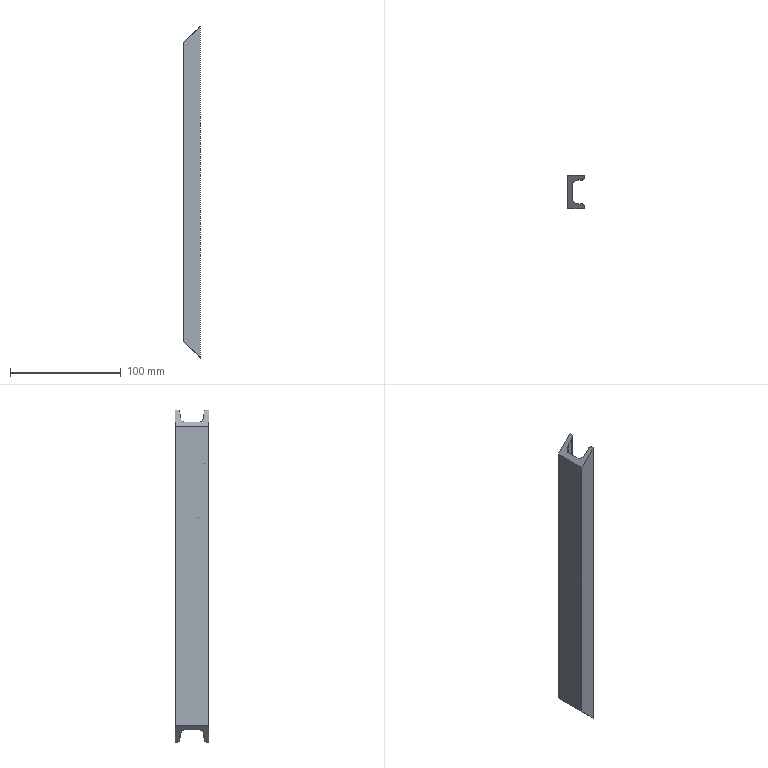Part | STEP file | DIN 1026-1 U 30x15 1785506933780 | 1 solid | 14 faces | box 15 x 30 x 300 mm | volume 62027 mm3 | plane 10 | cylinder 4 | commonest cylinder face diameters 4 x2 9 x2
STEP:
#1=CARTESIAN_POINT('',(13.159,-10.953,283.159));
#2=VERTEX_POINT('',#1);
#3=CARTESIAN_POINT('',(15.,-12.946,285.));
#4=VERTEX_POINT('',#3);
#5=CARTESIAN_POINT('',(13.,-12.946,283.));
#6=DIRECTION('',(0.7071,0.,-0.7071));
#7=DIRECTION('',(-0.7071,0.,-0.7071));
#8=AXIS2_PLACEMENT_3D('',#5,#6,#7);
#9=ELLIPSE('',#8,2.828,2.);
#10=EDGE_CURVE('',#2,#4,#9,.T.);
#11=ORIENTED_EDGE('',*,*,#10,.F.);
#12=CARTESIAN_POINT('',(8.141,-10.551,278.141));
#13=VERTEX_POINT('',#12);
#14=CARTESIAN_POINT('',(-132.725,0.718,137.275));
#15=DIRECTION('',(0.706,-0.05648,0.706));
#16=VECTOR('',#15,10.);
#17=LINE('',#14,#16);
#18=EDGE_CURVE('',#13,#2,#17,.T.);
#19=ORIENTED_EDGE('',*,*,#18,.F.);
#20=CARTESIAN_POINT('',(4.,-6.066,274.));
#21=VERTEX_POINT('',#20);
#22=CARTESIAN_POINT('',(8.5,-6.066,278.5));
#23=DIRECTION('',(-0.7071,0.,0.7071));
#24=DIRECTION('',(-0.7071,0.,-0.7071));
#25=AXIS2_PLACEMENT_3D('',#22,#23,#24);
#26=ELLIPSE('',#25,6.364,4.5);
#27=EDGE_CURVE('',#21,#13,#26,.T.);
#28=ORIENTED_EDGE('',*,*,#27,.F.);
#29=CARTESIAN_POINT('',(4.,6.066,274.));
#30=VERTEX_POINT('',#29);
#31=CARTESIAN_POINT('',(4.,0.,274.));
#32=DIRECTION('',(0.,-1.,0.));
#33=VECTOR('',#32,10.);
#34=LINE('',#31,#33);
#35=EDGE_CURVE('',#30,#21,#34,.T.);
#36=ORIENTED_EDGE('',*,*,#35,.F.);
#37=CARTESIAN_POINT('',(8.141,10.551,278.141));
#38=VERTEX_POINT('',#37);
#39=CARTESIAN_POINT('',(8.5,6.066,278.5));
#40=DIRECTION('',(-0.7071,0.,0.7071));
#41=DIRECTION('',(-0.7071,0.,-0.7071));
#42=AXIS2_PLACEMENT_3D('',#39,#40,#41);
#43=ELLIPSE('',#42,6.364,4.5);
#44=EDGE_CURVE('',#38,#30,#43,.T.);
#45=ORIENTED_EDGE('',*,*,#44,.F.);
#46=CARTESIAN_POINT('',(13.159,10.953,283.159));
#47=VERTEX_POINT('',#46);
#48=CARTESIAN_POINT('',(-131.466,-0.6173,138.534));
#49=DIRECTION('',(-0.706,-0.05648,-0.706));
#50=VECTOR('',#49,10.);
#51=LINE('',#48,#50);
#52=EDGE_CURVE('',#47,#38,#51,.T.);
#53=ORIENTED_EDGE('',*,*,#52,.F.);
#54=CARTESIAN_POINT('',(15.,12.946,285.));
#55=VERTEX_POINT('',#54);
#56=CARTESIAN_POINT('',(13.,12.946,283.));
#57=DIRECTION('',(0.7071,0.,-0.7071));
#58=DIRECTION('',(-0.7071,0.,-0.7071));
#59=AXIS2_PLACEMENT_3D('',#56,#57,#58);
#60=ELLIPSE('',#59,2.828,2.);
#61=EDGE_CURVE('',#55,#47,#60,.T.);
#62=ORIENTED_EDGE('',*,*,#61,.F.);
#63=CARTESIAN_POINT('',(15.,15.,285.));
#64=VERTEX_POINT('',#63);
#65=CARTESIAN_POINT('',(15.,7.5,285.));
#66=DIRECTION('',(0.,-1.,0.));
#67=VECTOR('',#66,10.);
#68=LINE('',#65,#67);
#69=EDGE_CURVE('',#64,#55,#68,.T.);
#70=ORIENTED_EDGE('',*,*,#69,.F.);
#71=CARTESIAN_POINT('',(0.,15.,270.));
#72=VERTEX_POINT('',#71);
#73=CARTESIAN_POINT('',(-135.,15.,135.));
#74=DIRECTION('',(0.7071,0.,0.7071));
#75=VECTOR('',#74,10.);
#76=LINE('',#73,#75);
#77=EDGE_CURVE('',#72,#64,#76,.T.);
#78=ORIENTED_EDGE('',*,*,#77,.F.);
#79=CARTESIAN_POINT('',(0.,-15.,270.));
#80=VERTEX_POINT('',#79);
#81=CARTESIAN_POINT('',(0.,0.,270.));
#82=DIRECTION('',(0.,1.,0.));
#83=VECTOR('',#82,10.);
#84=LINE('',#81,#83);
#85=EDGE_CURVE('',#80,#72,#84,.T.);
#86=ORIENTED_EDGE('',*,*,#85,.F.);
#87=CARTESIAN_POINT('',(15.,-15.,285.));
#88=VERTEX_POINT('',#87);
#89=CARTESIAN_POINT('',(-131.25,-15.,138.75));
#90=DIRECTION('',(-0.7071,0.,-0.7071));
#91=VECTOR('',#90,10.);
#92=LINE('',#89,#91);
#93=EDGE_CURVE('',#88,#80,#92,.T.);
#94=ORIENTED_EDGE('',*,*,#93,.F.);
#95=CARTESIAN_POINT('',(15.,-6.473,285.));
#96=DIRECTION('',(0.,-1.,0.));
#97=VECTOR('',#96,10.);
#98=LINE('',#95,#97);
#99=EDGE_CURVE('',#4,#88,#98,.T.);
#100=ORIENTED_EDGE('',*,*,#99,.F.);
#101=EDGE_LOOP('',(#11,#19,#28,#36,#45,#53,#62,#70,#78,#86,#94,#100));
#102=FACE_OUTER_BOUND('',#101,.T.);
#103=CARTESIAN_POINT('',(-135.,0.,135.));
#104=DIRECTION('',(0.7071,0.,-0.7071));
#105=DIRECTION('',(-0.7071,0.,-0.7071));
#106=AXIS2_PLACEMENT_3D('',#103,#104,#105);
#107=PLANE('',#106);
#108=ADVANCED_FACE('',(#102),#107,.F.);
#109=ORIENTED_EDGE('',*,*,#61,.T.);
#110=CARTESIAN_POINT('',(13.159,10.953,-13.159));
#111=VERTEX_POINT('',#110);
#112=CARTESIAN_POINT('',(13.159,10.953,0.));
#113=DIRECTION('',(0.,0.,-1.));
#114=VECTOR('',#113,10.);
#115=LINE('',#112,#114);
#116=EDGE_CURVE('',#47,#111,#115,.T.);
#117=ORIENTED_EDGE('',*,*,#116,.T.);
#118=CARTESIAN_POINT('',(15.,12.946,-15.));
#119=VERTEX_POINT('',#118);
#120=CARTESIAN_POINT('',(13.,12.946,-13.));
#121=DIRECTION('',(0.7071,0.,0.7071));
#122=DIRECTION('',(-0.7071,0.,0.7071));
#123=AXIS2_PLACEMENT_3D('',#120,#121,#122);
#124=ELLIPSE('',#123,2.828,2.);
#125=EDGE_CURVE('',#111,#119,#124,.T.);
#126=ORIENTED_EDGE('',*,*,#125,.T.);
#127=CARTESIAN_POINT('',(15.,12.946,0.));
#128=DIRECTION('',(0.,0.,-1.));
#129=VECTOR('',#128,10.);
#130=LINE('',#127,#129);
#131=EDGE_CURVE('',#55,#119,#130,.T.);
#132=ORIENTED_EDGE('',*,*,#131,.F.);
#133=EDGE_LOOP('',(#109,#117,#126,#132));
#134=FACE_OUTER_BOUND('',#133,.T.);
#135=CARTESIAN_POINT('',(13.,12.946,0.));
#136=DIRECTION('',(0.,0.,1.));
#137=DIRECTION('',(-0.07975,0.9968,0.));
#138=AXIS2_PLACEMENT_3D('',#135,#136,#137);
#139=CYLINDRICAL_SURFACE('',#138,2.);
#140=ADVANCED_FACE('',(#134),#139,.T.);
#141=ORIENTED_EDGE('',*,*,#52,.T.);
#142=CARTESIAN_POINT('',(8.141,10.551,-8.141));
#143=VERTEX_POINT('',#142);
#144=CARTESIAN_POINT('',(8.141,10.551,0.));
#145=DIRECTION('',(0.,0.,-1.));
#146=VECTOR('',#145,10.);
#147=LINE('',#144,#146);
#148=EDGE_CURVE('',#38,#143,#147,.T.);
#149=ORIENTED_EDGE('',*,*,#148,.T.);
#150=CARTESIAN_POINT('',(3.103,10.148,-3.103));
#151=DIRECTION('',(0.706,0.05648,-0.706));
#152=VECTOR('',#151,10.);
#153=LINE('',#150,#152);
#154=EDGE_CURVE('',#143,#111,#153,.T.);
#155=ORIENTED_EDGE('',*,*,#154,.T.);
#156=ORIENTED_EDGE('',*,*,#116,.F.);
#157=EDGE_LOOP('',(#141,#149,#155,#156));
#158=FACE_OUTER_BOUND('',#157,.T.);
#159=CARTESIAN_POINT('',(13.159,10.953,0.));
#160=DIRECTION('',(0.07975,-0.9968,0.));
#161=DIRECTION('',(0.,0.,-1.));
#162=AXIS2_PLACEMENT_3D('',#159,#160,#161);
#163=PLANE('',#162);
#164=ADVANCED_FACE('',(#158),#163,.T.);
#165=ORIENTED_EDGE('',*,*,#44,.T.);
#166=CARTESIAN_POINT('',(4.,6.066,-4.));
#167=VERTEX_POINT('',#166);
#168=CARTESIAN_POINT('',(4.,6.066,0.));
#169=DIRECTION('',(0.,0.,-1.));
#170=VECTOR('',#169,10.);
#171=LINE('',#168,#170);
#172=EDGE_CURVE('',#30,#167,#171,.T.);
#173=ORIENTED_EDGE('',*,*,#172,.T.);
#174=CARTESIAN_POINT('',(8.5,6.066,-8.5));
#175=DIRECTION('',(-0.7071,0.,-0.7071));
#176=DIRECTION('',(-0.7071,0.,0.7071));
#177=AXIS2_PLACEMENT_3D('',#174,#175,#176);
#178=ELLIPSE('',#177,6.364,4.5);
#179=EDGE_CURVE('',#167,#143,#178,.T.);
#180=ORIENTED_EDGE('',*,*,#179,.T.);
#181=ORIENTED_EDGE('',*,*,#148,.F.);
#182=EDGE_LOOP('',(#165,#173,#180,#181));
#183=FACE_OUTER_BOUND('',#182,.T.);
#184=CARTESIAN_POINT('',(8.5,6.066,0.));
#185=DIRECTION('',(0.,0.,1.));
#186=DIRECTION('',(-0.07975,0.9968,0.));
#187=AXIS2_PLACEMENT_3D('',#184,#185,#186);
#188=CYLINDRICAL_SURFACE('',#187,4.5);
#189=ADVANCED_FACE('',(#183),#188,.F.);
#190=ORIENTED_EDGE('',*,*,#35,.T.);
#191=CARTESIAN_POINT('',(4.,-6.066,-4.));
#192=VERTEX_POINT('',#191);
#193=CARTESIAN_POINT('',(4.,-6.066,0.));
#194=DIRECTION('',(0.,0.,-1.));
#195=VECTOR('',#194,10.);
#196=LINE('',#193,#195);
#197=EDGE_CURVE('',#21,#192,#196,.T.);
#198=ORIENTED_EDGE('',*,*,#197,.T.);
#199=CARTESIAN_POINT('',(4.,0.,-4.));
#200=DIRECTION('',(0.,1.,0.));
#201=VECTOR('',#200,10.);
#202=LINE('',#199,#201);
#203=EDGE_CURVE('',#192,#167,#202,.T.);
#204=ORIENTED_EDGE('',*,*,#203,.T.);
#205=ORIENTED_EDGE('',*,*,#172,.F.);
#206=EDGE_LOOP('',(#190,#198,#204,#205));
#207=FACE_OUTER_BOUND('',#206,.T.);
#208=CARTESIAN_POINT('',(4.,0.,0.));
#209=DIRECTION('',(1.,0.,0.));
#210=DIRECTION('',(0.,0.,-1.));
#211=AXIS2_PLACEMENT_3D('',#208,#209,#210);
#212=PLANE('',#211);
#213=ADVANCED_FACE('',(#207),#212,.T.);
#214=ORIENTED_EDGE('',*,*,#27,.T.);
#215=CARTESIAN_POINT('',(8.141,-10.551,-8.141));
#216=VERTEX_POINT('',#215);
#217=CARTESIAN_POINT('',(8.141,-10.551,0.));
#218=DIRECTION('',(0.,0.,-1.));
#219=VECTOR('',#218,10.);
#220=LINE('',#217,#219);
#221=EDGE_CURVE('',#13,#216,#220,.T.);
#222=ORIENTED_EDGE('',*,*,#221,.T.);
#223=CARTESIAN_POINT('',(8.5,-6.066,-8.5));
#224=DIRECTION('',(-0.7071,0.,-0.7071));
#225=DIRECTION('',(-0.7071,0.,0.7071));
#226=AXIS2_PLACEMENT_3D('',#223,#224,#225);
#227=ELLIPSE('',#226,6.364,4.5);
#228=EDGE_CURVE('',#216,#192,#227,.T.);
#229=ORIENTED_EDGE('',*,*,#228,.T.);
#230=ORIENTED_EDGE('',*,*,#197,.F.);
#231=EDGE_LOOP('',(#214,#222,#229,#230));
#232=FACE_OUTER_BOUND('',#231,.T.);
#233=CARTESIAN_POINT('',(8.5,-6.066,0.));
#234=DIRECTION('',(0.,0.,1.));
#235=DIRECTION('',(-1.,0.,0.));
#236=AXIS2_PLACEMENT_3D('',#233,#234,#235);
#237=CYLINDRICAL_SURFACE('',#236,4.5);
#238=ADVANCED_FACE('',(#232),#237,.F.);
#239=ORIENTED_EDGE('',*,*,#18,.T.);
#240=CARTESIAN_POINT('',(13.159,-10.953,-13.159));
#241=VERTEX_POINT('',#240);
#242=CARTESIAN_POINT('',(13.159,-10.953,0.));
#243=DIRECTION('',(0.,0.,-1.));
#244=VECTOR('',#243,10.);
#245=LINE('',#242,#244);
#246=EDGE_CURVE('',#2,#241,#245,.T.);
#247=ORIENTED_EDGE('',*,*,#246,.T.);
#248=CARTESIAN_POINT('',(1.844,-10.048,-1.844));
#249=DIRECTION('',(-0.706,0.05648,0.706));
#250=VECTOR('',#249,10.);
#251=LINE('',#248,#250);
#252=EDGE_CURVE('',#241,#216,#251,.T.);
#253=ORIENTED_EDGE('',*,*,#252,.T.);
#254=ORIENTED_EDGE('',*,*,#221,.F.);
#255=EDGE_LOOP('',(#239,#247,#253,#254));
#256=FACE_OUTER_BOUND('',#255,.T.);
#257=CARTESIAN_POINT('',(8.141,-10.551,0.));
#258=DIRECTION('',(0.07975,0.9968,0.));
#259=DIRECTION('',(0.,0.,1.));
#260=AXIS2_PLACEMENT_3D('',#257,#258,#259);
#261=PLANE('',#260);
#262=ADVANCED_FACE('',(#256),#261,.T.);
#263=ORIENTED_EDGE('',*,*,#228,.F.);
#264=ORIENTED_EDGE('',*,*,#252,.F.);
#265=CARTESIAN_POINT('',(15.,-12.946,-15.));
#266=VERTEX_POINT('',#265);
#267=CARTESIAN_POINT('',(13.,-12.946,-13.));
#268=DIRECTION('',(0.7071,0.,0.7071));
#269=DIRECTION('',(-0.7071,0.,0.7071));
#270=AXIS2_PLACEMENT_3D('',#267,#268,#269);
#271=ELLIPSE('',#270,2.828,2.);
#272=EDGE_CURVE('',#266,#241,#271,.T.);
#273=ORIENTED_EDGE('',*,*,#272,.F.);
#274=CARTESIAN_POINT('',(15.,-15.,-15.));
#275=VERTEX_POINT('',#274);
#276=CARTESIAN_POINT('',(15.,-6.473,-15.));
#277=DIRECTION('',(0.,-1.,0.));
#278=VECTOR('',#277,10.);
#279=LINE('',#276,#278);
#280=EDGE_CURVE('',#266,#275,#279,.T.);
#281=ORIENTED_EDGE('',*,*,#280,.T.);
#282=CARTESIAN_POINT('',(0.,-15.,0.));
#283=VERTEX_POINT('',#282);
#284=CARTESIAN_POINT('',(3.75,-15.,-3.75));
#285=DIRECTION('',(0.7071,0.,-0.7071));
#286=VECTOR('',#285,10.);
#287=LINE('',#284,#286);
#288=EDGE_CURVE('',#283,#275,#287,.T.);
#289=ORIENTED_EDGE('',*,*,#288,.F.);
#290=CARTESIAN_POINT('',(0.,15.,0.));
#291=VERTEX_POINT('',#290);
#292=CARTESIAN_POINT('',(0.,0.,0.));
#293=DIRECTION('',(0.,-1.,0.));
#294=VECTOR('',#293,10.);
#295=LINE('',#292,#294);
#296=EDGE_CURVE('',#291,#283,#295,.T.);
#297=ORIENTED_EDGE('',*,*,#296,.F.);
#298=CARTESIAN_POINT('',(15.,15.,-15.));
#299=VERTEX_POINT('',#298);
#300=CARTESIAN_POINT('',(0.,15.,0.));
#301=DIRECTION('',(-0.7071,0.,0.7071));
#302=VECTOR('',#301,10.);
#303=LINE('',#300,#302);
#304=EDGE_CURVE('',#299,#291,#303,.T.);
#305=ORIENTED_EDGE('',*,*,#304,.F.);
#306=CARTESIAN_POINT('',(15.,7.5,-15.));
#307=DIRECTION('',(0.,-1.,0.));
#308=VECTOR('',#307,10.);
#309=LINE('',#306,#308);
#310=EDGE_CURVE('',#299,#119,#309,.T.);
#311=ORIENTED_EDGE('',*,*,#310,.T.);
#312=ORIENTED_EDGE('',*,*,#125,.F.);
#313=ORIENTED_EDGE('',*,*,#154,.F.);
#314=ORIENTED_EDGE('',*,*,#179,.F.);
#315=ORIENTED_EDGE('',*,*,#203,.F.);
#316=EDGE_LOOP('',(#263,#264,#273,#281,#289,#297,#305,#311,#312,#313,#314,#315));
#317=FACE_OUTER_BOUND('',#316,.T.);
#318=CARTESIAN_POINT('',(0.,0.,0.));
#319=DIRECTION('',(0.7071,0.,0.7071));
#320=DIRECTION('',(0.7071,0.,-0.7071));
#321=AXIS2_PLACEMENT_3D('',#318,#319,#320);
#322=PLANE('',#321);
#323=ADVANCED_FACE('',(#317),#322,.F.);
#324=ORIENTED_EDGE('',*,*,#77,.T.);
#325=CARTESIAN_POINT('',(15.,15.,0.));
#326=DIRECTION('',(0.,0.,-1.));
#327=VECTOR('',#326,10.);
#328=LINE('',#325,#327);
#329=EDGE_CURVE('',#64,#299,#328,.T.);
#330=ORIENTED_EDGE('',*,*,#329,.T.);
#331=ORIENTED_EDGE('',*,*,#304,.T.);
#332=CARTESIAN_POINT('',(0.,15.,0.));
#333=DIRECTION('',(0.,0.,-1.));
#334=VECTOR('',#333,10.);
#335=LINE('',#332,#334);
#336=EDGE_CURVE('',#72,#291,#335,.T.);
#337=ORIENTED_EDGE('',*,*,#336,.F.);
#338=EDGE_LOOP('',(#324,#330,#331,#337));
#339=FACE_OUTER_BOUND('',#338,.T.);
#340=CARTESIAN_POINT('',(0.,15.,0.));
#341=DIRECTION('',(0.,1.,0.));
#342=DIRECTION('',(0.,0.,1.));
#343=AXIS2_PLACEMENT_3D('',#340,#341,#342);
#344=PLANE('',#343);
#345=ADVANCED_FACE('',(#339),#344,.T.);
#346=ORIENTED_EDGE('',*,*,#85,.T.);
#347=ORIENTED_EDGE('',*,*,#336,.T.);
#348=ORIENTED_EDGE('',*,*,#296,.T.);
#349=CARTESIAN_POINT('',(0.,-15.,0.));
#350=DIRECTION('',(0.,0.,-1.));
#351=VECTOR('',#350,10.);
#352=LINE('',#349,#351);
#353=EDGE_CURVE('',#80,#283,#352,.T.);
#354=ORIENTED_EDGE('',*,*,#353,.F.);
#355=EDGE_LOOP('',(#346,#347,#348,#354));
#356=FACE_OUTER_BOUND('',#355,.T.);
#357=CARTESIAN_POINT('',(0.,0.,0.));
#358=DIRECTION('',(-1.,0.,0.));
#359=DIRECTION('',(0.,0.,1.));
#360=AXIS2_PLACEMENT_3D('',#357,#358,#359);
#361=PLANE('',#360);
#362=ADVANCED_FACE('',(#356),#361,.T.);
#363=ORIENTED_EDGE('',*,*,#93,.T.);
#364=ORIENTED_EDGE('',*,*,#353,.T.);
#365=ORIENTED_EDGE('',*,*,#288,.T.);
#366=CARTESIAN_POINT('',(15.,-15.,0.));
#367=DIRECTION('',(0.,0.,-1.));
#368=VECTOR('',#367,10.);
#369=LINE('',#366,#368);
#370=EDGE_CURVE('',#88,#275,#369,.T.);
#371=ORIENTED_EDGE('',*,*,#370,.F.);
#372=EDGE_LOOP('',(#363,#364,#365,#371));
#373=FACE_OUTER_BOUND('',#372,.T.);
#374=CARTESIAN_POINT('',(15.,-15.,0.));
#375=DIRECTION('',(0.,-1.,0.));
#376=DIRECTION('',(0.,0.,-1.));
#377=AXIS2_PLACEMENT_3D('',#374,#375,#376);
#378=PLANE('',#377);
#379=ADVANCED_FACE('',(#373),#378,.T.);
#380=ORIENTED_EDGE('',*,*,#10,.T.);
#381=CARTESIAN_POINT('',(15.,-12.946,0.));
#382=DIRECTION('',(0.,0.,-1.));
#383=VECTOR('',#382,10.);
#384=LINE('',#381,#383);
#385=EDGE_CURVE('',#4,#266,#384,.T.);
#386=ORIENTED_EDGE('',*,*,#385,.T.);
#387=ORIENTED_EDGE('',*,*,#272,.T.);
#388=ORIENTED_EDGE('',*,*,#246,.F.);
#389=EDGE_LOOP('',(#380,#386,#387,#388));
#390=FACE_OUTER_BOUND('',#389,.T.);
#391=CARTESIAN_POINT('',(13.,-12.946,0.));
#392=DIRECTION('',(0.,0.,1.));
#393=DIRECTION('',(-1.,0.,0.));
#394=AXIS2_PLACEMENT_3D('',#391,#392,#393);
#395=CYLINDRICAL_SURFACE('',#394,2.);
#396=ADVANCED_FACE('',(#390),#395,.T.);
#397=ORIENTED_EDGE('',*,*,#99,.T.);
#398=ORIENTED_EDGE('',*,*,#370,.T.);
#399=ORIENTED_EDGE('',*,*,#280,.F.);
#400=ORIENTED_EDGE('',*,*,#385,.F.);
#401=EDGE_LOOP('',(#397,#398,#399,#400));
#402=FACE_OUTER_BOUND('',#401,.T.);
#403=CARTESIAN_POINT('',(15.,-12.946,0.));
#404=DIRECTION('',(1.,0.,0.));
#405=DIRECTION('',(0.,0.,-1.));
#406=AXIS2_PLACEMENT_3D('',#403,#404,#405);
#407=PLANE('',#406);
#408=ADVANCED_FACE('',(#402),#407,.T.);
#409=ORIENTED_EDGE('',*,*,#69,.T.);
#410=ORIENTED_EDGE('',*,*,#131,.T.);
#411=ORIENTED_EDGE('',*,*,#310,.F.);
#412=ORIENTED_EDGE('',*,*,#329,.F.);
#413=EDGE_LOOP('',(#409,#410,#411,#412));
#414=FACE_OUTER_BOUND('',#413,.T.);
#415=CARTESIAN_POINT('',(15.,15.,0.));
#416=DIRECTION('',(1.,0.,0.));
#417=DIRECTION('',(0.,0.,-1.));
#418=AXIS2_PLACEMENT_3D('',#415,#416,#417);
#419=PLANE('',#418);
#420=ADVANCED_FACE('',(#414),#419,.T.);
#421=CLOSED_SHELL('',(#108,#140,#164,#189,#213,#238,#262,#323,#345,#362,#379,#396,#408,#420));
#422=MANIFOLD_SOLID_BREP('',#421);
#423=(LENGTH_UNIT()NAMED_UNIT(*)SI_UNIT(.MILLI.,.METRE.));
#424=UNCERTAINTY_MEASURE_WITH_UNIT(LENGTH_MEASURE(0.01),#423,'','');
#425=(NAMED_UNIT(*)PLANE_ANGLE_UNIT()SI_UNIT($,.RADIAN.));
#426=(NAMED_UNIT(*)SI_UNIT($,.STERADIAN.)SOLID_ANGLE_UNIT());
#427=(GEOMETRIC_REPRESENTATION_CONTEXT(3)GLOBAL_UNCERTAINTY_ASSIGNED_CONTEXT((#424))GLOBAL_UNIT_ASSIGNED_CONTEXT((#423,#425,#426))REPRESENTATION_CONTEXT('',''));
#428=ADVANCED_BREP_SHAPE_REPRESENTATION('',(#422),#427);